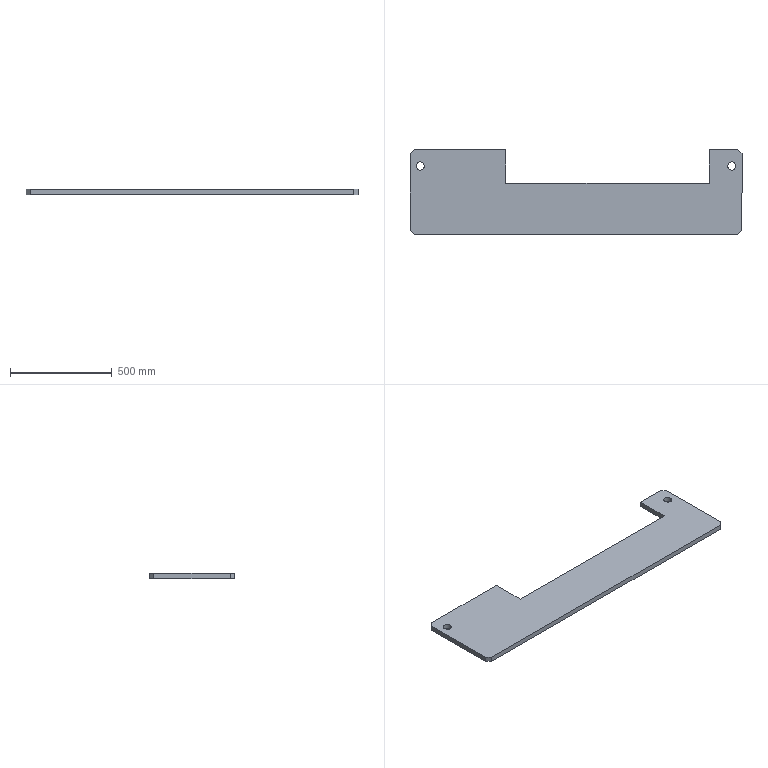Part | SolidWorks | features Chamfer 1, Extrusion 1, ICE 1 | 1 solid | 18 faces | box 1630 x 415 x 25 mm | volume 12703418 mm3 | plane 14 | cylinder 4 | commonest cylinder face diameters 40 x4
STEP:
#1=CARTESIAN_POINT('',(745.,127.5,0.));
#2=VERTEX_POINT('',#1);
#3=CARTESIAN_POINT('',(785.,127.5,0.));
#4=VERTEX_POINT('',#3);
#5=CARTESIAN_POINT('',(765.,127.5,0.));
#6=DIRECTION('',(0.,0.,1.));
#7=DIRECTION('',(1.,0.,0.));
#8=AXIS2_PLACEMENT_3D('',#5,#6,#7);
#9=CIRCLE('',#8,20.);
#10=EDGE_CURVE('',#2,#4,#9,.T.);
#11=ORIENTED_EDGE('',*,*,#10,.F.);
#12=CARTESIAN_POINT('',(745.,127.5,25.));
#13=VERTEX_POINT('',#12);
#14=CARTESIAN_POINT('',(745.,127.5,0.));
#15=DIRECTION('',(0.,0.,1.));
#16=VECTOR('',#15,1000.);
#17=LINE('',#14,#16);
#18=EDGE_CURVE('',#2,#13,#17,.T.);
#19=ORIENTED_EDGE('',*,*,#18,.T.);
#20=CARTESIAN_POINT('',(785.,127.5,25.));
#21=VERTEX_POINT('',#20);
#22=CARTESIAN_POINT('',(765.,127.5,25.));
#23=DIRECTION('',(0.,0.,-1.));
#24=DIRECTION('',(-1.,0.,0.));
#25=AXIS2_PLACEMENT_3D('',#22,#23,#24);
#26=CIRCLE('',#25,20.);
#27=EDGE_CURVE('',#21,#13,#26,.T.);
#28=ORIENTED_EDGE('',*,*,#27,.F.);
#29=CARTESIAN_POINT('',(785.,127.5,0.));
#30=DIRECTION('',(0.,0.,1.));
#31=VECTOR('',#30,1000.);
#32=LINE('',#29,#31);
#33=EDGE_CURVE('',#4,#21,#32,.T.);
#34=ORIENTED_EDGE('',*,*,#33,.F.);
#35=EDGE_LOOP('',(#11,#19,#28,#34));
#36=FACE_OUTER_BOUND('',#35,.T.);
#37=CARTESIAN_POINT('',(765.,127.5,0.));
#38=DIRECTION('',(0.,0.,1.));
#39=DIRECTION('',(1.,0.,0.));
#40=AXIS2_PLACEMENT_3D('',#37,#38,#39);
#41=CYLINDRICAL_SURFACE('',#40,20.);
#42=ADVANCED_FACE('',(#36),#41,.F.);
#43=CARTESIAN_POINT('',(-785.,127.5,0.));
#44=VERTEX_POINT('',#43);
#45=CARTESIAN_POINT('',(-745.,127.5,0.));
#46=VERTEX_POINT('',#45);
#47=CARTESIAN_POINT('',(-765.,127.5,0.));
#48=DIRECTION('',(0.,0.,1.));
#49=DIRECTION('',(1.,0.,0.));
#50=AXIS2_PLACEMENT_3D('',#47,#48,#49);
#51=CIRCLE('',#50,20.);
#52=EDGE_CURVE('',#44,#46,#51,.T.);
#53=ORIENTED_EDGE('',*,*,#52,.F.);
#54=CARTESIAN_POINT('',(-785.,127.5,25.));
#55=VERTEX_POINT('',#54);
#56=CARTESIAN_POINT('',(-785.,127.5,0.));
#57=DIRECTION('',(0.,0.,1.));
#58=VECTOR('',#57,1000.);
#59=LINE('',#56,#58);
#60=EDGE_CURVE('',#44,#55,#59,.T.);
#61=ORIENTED_EDGE('',*,*,#60,.T.);
#62=CARTESIAN_POINT('',(-745.,127.5,25.));
#63=VERTEX_POINT('',#62);
#64=CARTESIAN_POINT('',(-765.,127.5,25.));
#65=DIRECTION('',(0.,0.,-1.));
#66=DIRECTION('',(-1.,0.,0.));
#67=AXIS2_PLACEMENT_3D('',#64,#65,#66);
#68=CIRCLE('',#67,20.);
#69=EDGE_CURVE('',#63,#55,#68,.T.);
#70=ORIENTED_EDGE('',*,*,#69,.F.);
#71=CARTESIAN_POINT('',(-745.,127.5,0.));
#72=DIRECTION('',(0.,0.,1.));
#73=VECTOR('',#72,1000.);
#74=LINE('',#71,#73);
#75=EDGE_CURVE('',#46,#63,#74,.T.);
#76=ORIENTED_EDGE('',*,*,#75,.F.);
#77=EDGE_LOOP('',(#53,#61,#70,#76));
#78=FACE_OUTER_BOUND('',#77,.T.);
#79=CARTESIAN_POINT('',(-765.,127.5,0.));
#80=DIRECTION('',(0.,0.,1.));
#81=DIRECTION('',(1.,0.,0.));
#82=AXIS2_PLACEMENT_3D('',#79,#80,#81);
#83=CYLINDRICAL_SURFACE('',#82,20.);
#84=ADVANCED_FACE('',(#78),#83,.F.);
#85=CARTESIAN_POINT('',(-345.,207.5,25.));
#86=VERTEX_POINT('',#85);
#87=CARTESIAN_POINT('',(-795.,207.5,25.));
#88=VERTEX_POINT('',#87);
#89=CARTESIAN_POINT('',(815.,207.5,25.));
#90=DIRECTION('',(-1.,0.,0.));
#91=VECTOR('',#90,1000.);
#92=LINE('',#89,#91);
#93=EDGE_CURVE('',#86,#88,#92,.T.);
#94=ORIENTED_EDGE('',*,*,#93,.F.);
#95=CARTESIAN_POINT('',(-345.,207.5,0.));
#96=VERTEX_POINT('',#95);
#97=CARTESIAN_POINT('',(-345.,207.5,25.));
#98=DIRECTION('',(0.,0.,-1.));
#99=VECTOR('',#98,1000.);
#100=LINE('',#97,#99);
#101=EDGE_CURVE('',#86,#96,#100,.T.);
#102=ORIENTED_EDGE('',*,*,#101,.T.);
#103=CARTESIAN_POINT('',(-795.,207.5,0.));
#104=VERTEX_POINT('',#103);
#105=CARTESIAN_POINT('',(815.,207.5,0.));
#106=DIRECTION('',(-1.,0.,0.));
#107=VECTOR('',#106,1000.);
#108=LINE('',#105,#107);
#109=EDGE_CURVE('',#96,#104,#108,.T.);
#110=ORIENTED_EDGE('',*,*,#109,.T.);
#111=CARTESIAN_POINT('',(-795.,207.5,25.));
#112=DIRECTION('',(0.,0.,1.));
#113=VECTOR('',#112,1000.);
#114=LINE('',#111,#113);
#115=EDGE_CURVE('',#104,#88,#114,.T.);
#116=ORIENTED_EDGE('',*,*,#115,.T.);
#117=EDGE_LOOP('',(#94,#102,#110,#116));
#118=FACE_OUTER_BOUND('',#117,.T.);
#119=CARTESIAN_POINT('',(815.,207.5,25.));
#120=DIRECTION('',(0.,-1.,0.));
#121=DIRECTION('',(1.,0.,0.));
#122=AXIS2_PLACEMENT_3D('',#119,#120,#121);
#123=PLANE('',#122);
#124=ADVANCED_FACE('',(#118),#123,.F.);
#125=CARTESIAN_POINT('',(-815.,187.5,0.));
#126=VERTEX_POINT('',#125);
#127=CARTESIAN_POINT('',(-815.,-187.5,0.));
#128=VERTEX_POINT('',#127);
#129=CARTESIAN_POINT('',(-815.,207.5,0.));
#130=DIRECTION('',(0.,-1.,0.));
#131=VECTOR('',#130,1000.);
#132=LINE('',#129,#131);
#133=EDGE_CURVE('',#126,#128,#132,.T.);
#134=ORIENTED_EDGE('',*,*,#133,.T.);
#135=CARTESIAN_POINT('',(-815.,-187.5,25.));
#136=VERTEX_POINT('',#135);
#137=CARTESIAN_POINT('',(-815.,-187.5,25.));
#138=DIRECTION('',(0.,0.,1.));
#139=VECTOR('',#138,1000.);
#140=LINE('',#137,#139);
#141=EDGE_CURVE('',#128,#136,#140,.T.);
#142=ORIENTED_EDGE('',*,*,#141,.T.);
#143=CARTESIAN_POINT('',(-815.,187.5,25.));
#144=VERTEX_POINT('',#143);
#145=CARTESIAN_POINT('',(-815.,207.5,25.));
#146=DIRECTION('',(0.,-1.,0.));
#147=VECTOR('',#146,1000.);
#148=LINE('',#145,#147);
#149=EDGE_CURVE('',#144,#136,#148,.T.);
#150=ORIENTED_EDGE('',*,*,#149,.F.);
#151=CARTESIAN_POINT('',(-815.,187.5,25.));
#152=DIRECTION('',(0.,0.,-1.));
#153=VECTOR('',#152,1000.);
#154=LINE('',#151,#153);
#155=EDGE_CURVE('',#144,#126,#154,.T.);
#156=ORIENTED_EDGE('',*,*,#155,.T.);
#157=EDGE_LOOP('',(#134,#142,#150,#156));
#158=FACE_OUTER_BOUND('',#157,.T.);
#159=CARTESIAN_POINT('',(-815.,207.5,25.));
#160=DIRECTION('',(1.,0.,0.));
#161=DIRECTION('',(0.,1.,0.));
#162=AXIS2_PLACEMENT_3D('',#159,#160,#161);
#163=PLANE('',#162);
#164=ADVANCED_FACE('',(#158),#163,.F.);
#165=CARTESIAN_POINT('',(-795.,-207.5,25.));
#166=VERTEX_POINT('',#165);
#167=CARTESIAN_POINT('',(795.,-207.5,25.));
#168=VERTEX_POINT('',#167);
#169=CARTESIAN_POINT('',(815.,-207.5,25.));
#170=DIRECTION('',(1.,0.,0.));
#171=VECTOR('',#170,1000.);
#172=LINE('',#169,#171);
#173=EDGE_CURVE('',#166,#168,#172,.T.);
#174=ORIENTED_EDGE('',*,*,#173,.F.);
#175=CARTESIAN_POINT('',(-795.,-207.5,0.));
#176=VERTEX_POINT('',#175);
#177=CARTESIAN_POINT('',(-795.,-207.5,25.));
#178=DIRECTION('',(0.,0.,-1.));
#179=VECTOR('',#178,1000.);
#180=LINE('',#177,#179);
#181=EDGE_CURVE('',#166,#176,#180,.T.);
#182=ORIENTED_EDGE('',*,*,#181,.T.);
#183=CARTESIAN_POINT('',(795.,-207.5,0.));
#184=VERTEX_POINT('',#183);
#185=CARTESIAN_POINT('',(815.,-207.5,0.));
#186=DIRECTION('',(1.,0.,0.));
#187=VECTOR('',#186,1000.);
#188=LINE('',#185,#187);
#189=EDGE_CURVE('',#176,#184,#188,.T.);
#190=ORIENTED_EDGE('',*,*,#189,.T.);
#191=CARTESIAN_POINT('',(795.,-207.5,25.));
#192=DIRECTION('',(0.,0.,1.));
#193=VECTOR('',#192,1000.);
#194=LINE('',#191,#193);
#195=EDGE_CURVE('',#184,#168,#194,.T.);
#196=ORIENTED_EDGE('',*,*,#195,.T.);
#197=EDGE_LOOP('',(#174,#182,#190,#196));
#198=FACE_OUTER_BOUND('',#197,.T.);
#199=CARTESIAN_POINT('',(815.,-207.5,25.));
#200=DIRECTION('',(0.,1.,0.));
#201=DIRECTION('',(-1.,0.,0.));
#202=AXIS2_PLACEMENT_3D('',#199,#200,#201);
#203=PLANE('',#202);
#204=ADVANCED_FACE('',(#198),#203,.F.);
#205=CARTESIAN_POINT('',(815.,-187.5,25.));
#206=VERTEX_POINT('',#205);
#207=CARTESIAN_POINT('',(815.,187.5,25.));
#208=VERTEX_POINT('',#207);
#209=CARTESIAN_POINT('',(815.,207.5,25.));
#210=DIRECTION('',(0.,1.,0.));
#211=VECTOR('',#210,1000.);
#212=LINE('',#209,#211);
#213=EDGE_CURVE('',#206,#208,#212,.T.);
#214=ORIENTED_EDGE('',*,*,#213,.F.);
#215=CARTESIAN_POINT('',(815.,-187.5,0.));
#216=VERTEX_POINT('',#215);
#217=CARTESIAN_POINT('',(815.,-187.5,25.));
#218=DIRECTION('',(0.,0.,-1.));
#219=VECTOR('',#218,1000.);
#220=LINE('',#217,#219);
#221=EDGE_CURVE('',#206,#216,#220,.T.);
#222=ORIENTED_EDGE('',*,*,#221,.T.);
#223=CARTESIAN_POINT('',(815.,187.5,0.));
#224=VERTEX_POINT('',#223);
#225=CARTESIAN_POINT('',(815.,207.5,0.));
#226=DIRECTION('',(0.,1.,0.));
#227=VECTOR('',#226,1000.);
#228=LINE('',#225,#227);
#229=EDGE_CURVE('',#216,#224,#228,.T.);
#230=ORIENTED_EDGE('',*,*,#229,.T.);
#231=CARTESIAN_POINT('',(815.,187.5,25.));
#232=DIRECTION('',(0.,0.,1.));
#233=VECTOR('',#232,1000.);
#234=LINE('',#231,#233);
#235=EDGE_CURVE('',#224,#208,#234,.T.);
#236=ORIENTED_EDGE('',*,*,#235,.T.);
#237=EDGE_LOOP('',(#214,#222,#230,#236));
#238=FACE_OUTER_BOUND('',#237,.T.);
#239=CARTESIAN_POINT('',(815.,207.5,25.));
#240=DIRECTION('',(-1.,0.,0.));
#241=DIRECTION('',(0.,-1.,0.));
#242=AXIS2_PLACEMENT_3D('',#239,#240,#241);
#243=PLANE('',#242);
#244=ADVANCED_FACE('',(#238),#243,.F.);
#245=CARTESIAN_POINT('',(795.,207.5,0.));
#246=VERTEX_POINT('',#245);
#247=CARTESIAN_POINT('',(655.,207.5,0.));
#248=VERTEX_POINT('',#247);
#249=CARTESIAN_POINT('',(815.,207.5,0.));
#250=DIRECTION('',(-1.,0.,0.));
#251=VECTOR('',#250,1000.);
#252=LINE('',#249,#251);
#253=EDGE_CURVE('',#246,#248,#252,.T.);
#254=ORIENTED_EDGE('',*,*,#253,.T.);
#255=CARTESIAN_POINT('',(655.,207.5,25.));
#256=VERTEX_POINT('',#255);
#257=CARTESIAN_POINT('',(655.,207.5,25.));
#258=DIRECTION('',(0.,0.,1.));
#259=VECTOR('',#258,1000.);
#260=LINE('',#257,#259);
#261=EDGE_CURVE('',#248,#256,#260,.T.);
#262=ORIENTED_EDGE('',*,*,#261,.T.);
#263=CARTESIAN_POINT('',(795.,207.5,25.));
#264=VERTEX_POINT('',#263);
#265=CARTESIAN_POINT('',(815.,207.5,25.));
#266=DIRECTION('',(-1.,0.,0.));
#267=VECTOR('',#266,1000.);
#268=LINE('',#265,#267);
#269=EDGE_CURVE('',#264,#256,#268,.T.);
#270=ORIENTED_EDGE('',*,*,#269,.F.);
#271=CARTESIAN_POINT('',(795.,207.5,25.));
#272=DIRECTION('',(0.,0.,-1.));
#273=VECTOR('',#272,1000.);
#274=LINE('',#271,#273);
#275=EDGE_CURVE('',#264,#246,#274,.T.);
#276=ORIENTED_EDGE('',*,*,#275,.T.);
#277=EDGE_LOOP('',(#254,#262,#270,#276));
#278=FACE_OUTER_BOUND('',#277,.T.);
#279=CARTESIAN_POINT('',(815.,207.5,25.));
#280=DIRECTION('',(0.,-1.,0.));
#281=DIRECTION('',(1.,0.,0.));
#282=AXIS2_PLACEMENT_3D('',#279,#280,#281);
#283=PLANE('',#282);
#284=ADVANCED_FACE('',(#278),#283,.F.);
#285=ORIENTED_EDGE('',*,*,#27,.T.);
#286=CARTESIAN_POINT('',(765.,127.5,25.));
#287=DIRECTION('',(0.,0.,-1.));
#288=DIRECTION('',(-1.,0.,0.));
#289=AXIS2_PLACEMENT_3D('',#286,#287,#288);
#290=CIRCLE('',#289,20.);
#291=EDGE_CURVE('',#13,#21,#290,.T.);
#292=ORIENTED_EDGE('',*,*,#291,.T.);
#293=EDGE_LOOP('',(#285,#292));
#294=FACE_BOUND('',#293,.T.);
#295=ORIENTED_EDGE('',*,*,#69,.T.);
#296=CARTESIAN_POINT('',(-765.,127.5,25.));
#297=DIRECTION('',(0.,0.,-1.));
#298=DIRECTION('',(-1.,0.,0.));
#299=AXIS2_PLACEMENT_3D('',#296,#297,#298);
#300=CIRCLE('',#299,20.);
#301=EDGE_CURVE('',#55,#63,#300,.T.);
#302=ORIENTED_EDGE('',*,*,#301,.T.);
#303=EDGE_LOOP('',(#295,#302));
#304=FACE_BOUND('',#303,.T.);
#305=CARTESIAN_POINT('',(655.,42.5,25.));
#306=VERTEX_POINT('',#305);
#307=CARTESIAN_POINT('',(-345.,42.5,25.));
#308=VERTEX_POINT('',#307);
#309=CARTESIAN_POINT('',(0.,42.5,25.));
#310=DIRECTION('',(-1.,0.,0.));
#311=VECTOR('',#310,1000.);
#312=LINE('',#309,#311);
#313=EDGE_CURVE('',#306,#308,#312,.T.);
#314=ORIENTED_EDGE('',*,*,#313,.T.);
#315=CARTESIAN_POINT('',(-345.,0.,25.));
#316=DIRECTION('',(0.,1.,0.));
#317=VECTOR('',#316,1000.);
#318=LINE('',#315,#317);
#319=EDGE_CURVE('',#308,#86,#318,.T.);
#320=ORIENTED_EDGE('',*,*,#319,.T.);
#321=ORIENTED_EDGE('',*,*,#93,.T.);
#322=CARTESIAN_POINT('',(-815.,187.5,25.));
#323=DIRECTION('',(-0.7071,-0.7071,0.));
#324=VECTOR('',#323,1000.);
#325=LINE('',#322,#324);
#326=EDGE_CURVE('',#88,#144,#325,.T.);
#327=ORIENTED_EDGE('',*,*,#326,.T.);
#328=ORIENTED_EDGE('',*,*,#149,.T.);
#329=CARTESIAN_POINT('',(-795.,-207.5,25.));
#330=DIRECTION('',(0.7071,-0.7071,0.));
#331=VECTOR('',#330,1000.);
#332=LINE('',#329,#331);
#333=EDGE_CURVE('',#136,#166,#332,.T.);
#334=ORIENTED_EDGE('',*,*,#333,.T.);
#335=ORIENTED_EDGE('',*,*,#173,.T.);
#336=CARTESIAN_POINT('',(815.,-187.5,25.));
#337=DIRECTION('',(0.7071,0.7071,0.));
#338=VECTOR('',#337,1000.);
#339=LINE('',#336,#338);
#340=EDGE_CURVE('',#168,#206,#339,.T.);
#341=ORIENTED_EDGE('',*,*,#340,.T.);
#342=ORIENTED_EDGE('',*,*,#213,.T.);
#343=CARTESIAN_POINT('',(795.,207.5,25.));
#344=DIRECTION('',(-0.7071,0.7071,0.));
#345=VECTOR('',#344,1000.);
#346=LINE('',#343,#345);
#347=EDGE_CURVE('',#208,#264,#346,.T.);
#348=ORIENTED_EDGE('',*,*,#347,.T.);
#349=ORIENTED_EDGE('',*,*,#269,.T.);
#350=CARTESIAN_POINT('',(655.,0.,25.));
#351=DIRECTION('',(0.,-1.,0.));
#352=VECTOR('',#351,1000.);
#353=LINE('',#350,#352);
#354=EDGE_CURVE('',#256,#306,#353,.T.);
#355=ORIENTED_EDGE('',*,*,#354,.T.);
#356=EDGE_LOOP('',(#314,#320,#321,#327,#328,#334,#335,#341,#342,#348,#349,#355));
#357=FACE_OUTER_BOUND('',#356,.T.);
#358=CARTESIAN_POINT('',(0.,0.,25.));
#359=DIRECTION('',(0.,0.,-1.));
#360=DIRECTION('',(-1.,0.,0.));
#361=AXIS2_PLACEMENT_3D('',#358,#359,#360);
#362=PLANE('',#361);
#363=ADVANCED_FACE('',(#294,#304,#357),#362,.F.);
#364=CARTESIAN_POINT('',(765.,127.5,0.));
#365=DIRECTION('',(0.,0.,1.));
#366=DIRECTION('',(1.,0.,0.));
#367=AXIS2_PLACEMENT_3D('',#364,#365,#366);
#368=CIRCLE('',#367,20.);
#369=EDGE_CURVE('',#4,#2,#368,.T.);
#370=ORIENTED_EDGE('',*,*,#369,.T.);
#371=ORIENTED_EDGE('',*,*,#10,.T.);
#372=EDGE_LOOP('',(#370,#371));
#373=FACE_BOUND('',#372,.T.);
#374=CARTESIAN_POINT('',(-765.,127.5,0.));
#375=DIRECTION('',(0.,0.,1.));
#376=DIRECTION('',(1.,0.,0.));
#377=AXIS2_PLACEMENT_3D('',#374,#375,#376);
#378=CIRCLE('',#377,20.);
#379=EDGE_CURVE('',#46,#44,#378,.T.);
#380=ORIENTED_EDGE('',*,*,#379,.T.);
#381=ORIENTED_EDGE('',*,*,#52,.T.);
#382=EDGE_LOOP('',(#380,#381));
#383=FACE_BOUND('',#382,.T.);
#384=CARTESIAN_POINT('',(-345.,42.5,0.));
#385=VERTEX_POINT('',#384);
#386=CARTESIAN_POINT('',(-345.,0.,0.));
#387=DIRECTION('',(0.,1.,0.));
#388=VECTOR('',#387,1000.);
#389=LINE('',#386,#388);
#390=EDGE_CURVE('',#385,#96,#389,.T.);
#391=ORIENTED_EDGE('',*,*,#390,.F.);
#392=CARTESIAN_POINT('',(655.,42.5,0.));
#393=VERTEX_POINT('',#392);
#394=CARTESIAN_POINT('',(-345.,42.5,0.));
#395=DIRECTION('',(1.,0.,0.));
#396=VECTOR('',#395,1000.);
#397=LINE('',#394,#396);
#398=EDGE_CURVE('',#385,#393,#397,.T.);
#399=ORIENTED_EDGE('',*,*,#398,.T.);
#400=CARTESIAN_POINT('',(655.,42.5,0.));
#401=DIRECTION('',(0.,1.,0.));
#402=VECTOR('',#401,1000.);
#403=LINE('',#400,#402);
#404=EDGE_CURVE('',#393,#248,#403,.T.);
#405=ORIENTED_EDGE('',*,*,#404,.T.);
#406=ORIENTED_EDGE('',*,*,#253,.F.);
#407=CARTESIAN_POINT('',(501.25,501.25,0.));
#408=DIRECTION('',(0.7071,-0.7071,0.));
#409=VECTOR('',#408,1000.);
#410=LINE('',#407,#409);
#411=EDGE_CURVE('',#246,#224,#410,.T.);
#412=ORIENTED_EDGE('',*,*,#411,.T.);
#413=ORIENTED_EDGE('',*,*,#229,.F.);
#414=CARTESIAN_POINT('',(501.25,-501.25,0.));
#415=DIRECTION('',(-0.7071,-0.7071,0.));
#416=VECTOR('',#415,1000.);
#417=LINE('',#414,#416);
#418=EDGE_CURVE('',#216,#184,#417,.T.);
#419=ORIENTED_EDGE('',*,*,#418,.T.);
#420=ORIENTED_EDGE('',*,*,#189,.F.);
#421=CARTESIAN_POINT('',(-501.25,-501.25,0.));
#422=DIRECTION('',(-0.7071,0.7071,0.));
#423=VECTOR('',#422,1000.);
#424=LINE('',#421,#423);
#425=EDGE_CURVE('',#176,#128,#424,.T.);
#426=ORIENTED_EDGE('',*,*,#425,.T.);
#427=ORIENTED_EDGE('',*,*,#133,.F.);
#428=CARTESIAN_POINT('',(-501.25,501.25,0.));
#429=DIRECTION('',(0.7071,0.7071,0.));
#430=VECTOR('',#429,1000.);
#431=LINE('',#428,#430);
#432=EDGE_CURVE('',#126,#104,#431,.T.);
#433=ORIENTED_EDGE('',*,*,#432,.T.);
#434=ORIENTED_EDGE('',*,*,#109,.F.);
#435=EDGE_LOOP('',(#391,#399,#405,#406,#412,#413,#419,#420,#426,#427,#433,#434));
#436=FACE_OUTER_BOUND('',#435,.T.);
#437=CARTESIAN_POINT('',(0.,0.,0.));
#438=DIRECTION('',(0.,0.,-1.));
#439=DIRECTION('',(-1.,0.,0.));
#440=AXIS2_PLACEMENT_3D('',#437,#438,#439);
#441=PLANE('',#440);
#442=ADVANCED_FACE('',(#373,#383,#436),#441,.T.);
#443=ORIENTED_EDGE('',*,*,#333,.F.);
#444=ORIENTED_EDGE('',*,*,#141,.F.);
#445=ORIENTED_EDGE('',*,*,#425,.F.);
#446=ORIENTED_EDGE('',*,*,#181,.F.);
#447=EDGE_LOOP('',(#443,#444,#445,#446));
#448=FACE_OUTER_BOUND('',#447,.T.);
#449=CARTESIAN_POINT('',(-795.,-207.5,25.));
#450=DIRECTION('',(0.7071,0.7071,0.));
#451=DIRECTION('',(0.,0.,-1.));
#452=AXIS2_PLACEMENT_3D('',#449,#450,#451);
#453=PLANE('',#452);
#454=ADVANCED_FACE('',(#448),#453,.F.);
#455=ORIENTED_EDGE('',*,*,#340,.F.);
#456=ORIENTED_EDGE('',*,*,#195,.F.);
#457=ORIENTED_EDGE('',*,*,#418,.F.);
#458=ORIENTED_EDGE('',*,*,#221,.F.);
#459=EDGE_LOOP('',(#455,#456,#457,#458));
#460=FACE_OUTER_BOUND('',#459,.T.);
#461=CARTESIAN_POINT('',(815.,-187.5,25.));
#462=DIRECTION('',(-0.7071,0.7071,0.));
#463=DIRECTION('',(0.,0.,-1.));
#464=AXIS2_PLACEMENT_3D('',#461,#462,#463);
#465=PLANE('',#464);
#466=ADVANCED_FACE('',(#460),#465,.F.);
#467=ORIENTED_EDGE('',*,*,#347,.F.);
#468=ORIENTED_EDGE('',*,*,#235,.F.);
#469=ORIENTED_EDGE('',*,*,#411,.F.);
#470=ORIENTED_EDGE('',*,*,#275,.F.);
#471=EDGE_LOOP('',(#467,#468,#469,#470));
#472=FACE_OUTER_BOUND('',#471,.T.);
#473=CARTESIAN_POINT('',(795.,207.5,25.));
#474=DIRECTION('',(-0.7071,-0.7071,0.));
#475=DIRECTION('',(0.,0.,-1.));
#476=AXIS2_PLACEMENT_3D('',#473,#474,#475);
#477=PLANE('',#476);
#478=ADVANCED_FACE('',(#472),#477,.F.);
#479=ORIENTED_EDGE('',*,*,#326,.F.);
#480=ORIENTED_EDGE('',*,*,#115,.F.);
#481=ORIENTED_EDGE('',*,*,#432,.F.);
#482=ORIENTED_EDGE('',*,*,#155,.F.);
#483=EDGE_LOOP('',(#479,#480,#481,#482));
#484=FACE_OUTER_BOUND('',#483,.T.);
#485=CARTESIAN_POINT('',(-815.,187.5,25.));
#486=DIRECTION('',(0.7071,-0.7071,0.));
#487=DIRECTION('',(0.,0.,-1.));
#488=AXIS2_PLACEMENT_3D('',#485,#486,#487);
#489=PLANE('',#488);
#490=ADVANCED_FACE('',(#484),#489,.F.);
#491=ORIENTED_EDGE('',*,*,#319,.F.);
#492=CARTESIAN_POINT('',(-345.,42.5,0.));
#493=DIRECTION('',(0.,0.,1.));
#494=VECTOR('',#493,1000.);
#495=LINE('',#492,#494);
#496=EDGE_CURVE('',#385,#308,#495,.T.);
#497=ORIENTED_EDGE('',*,*,#496,.F.);
#498=ORIENTED_EDGE('',*,*,#390,.T.);
#499=ORIENTED_EDGE('',*,*,#101,.F.);
#500=EDGE_LOOP('',(#491,#497,#498,#499));
#501=FACE_OUTER_BOUND('',#500,.T.);
#502=CARTESIAN_POINT('',(-345.,42.5,0.));
#503=DIRECTION('',(-1.,0.,0.));
#504=DIRECTION('',(0.,0.,1.));
#505=AXIS2_PLACEMENT_3D('',#502,#503,#504);
#506=PLANE('',#505);
#507=ADVANCED_FACE('',(#501),#506,.F.);
#508=ORIENTED_EDGE('',*,*,#404,.F.);
#509=CARTESIAN_POINT('',(655.,42.5,0.));
#510=DIRECTION('',(0.,0.,1.));
#511=VECTOR('',#510,1000.);
#512=LINE('',#509,#511);
#513=EDGE_CURVE('',#393,#306,#512,.T.);
#514=ORIENTED_EDGE('',*,*,#513,.T.);
#515=ORIENTED_EDGE('',*,*,#354,.F.);
#516=ORIENTED_EDGE('',*,*,#261,.F.);
#517=EDGE_LOOP('',(#508,#514,#515,#516));
#518=FACE_OUTER_BOUND('',#517,.T.);
#519=CARTESIAN_POINT('',(655.,42.5,0.));
#520=DIRECTION('',(1.,0.,0.));
#521=DIRECTION('',(0.,0.,-1.));
#522=AXIS2_PLACEMENT_3D('',#519,#520,#521);
#523=PLANE('',#522);
#524=ADVANCED_FACE('',(#518),#523,.F.);
#525=ORIENTED_EDGE('',*,*,#513,.F.);
#526=ORIENTED_EDGE('',*,*,#398,.F.);
#527=ORIENTED_EDGE('',*,*,#496,.T.);
#528=ORIENTED_EDGE('',*,*,#313,.F.);
#529=EDGE_LOOP('',(#525,#526,#527,#528));
#530=FACE_OUTER_BOUND('',#529,.T.);
#531=CARTESIAN_POINT('',(-345.,42.5,0.));
#532=DIRECTION('',(0.,-1.,0.));
#533=DIRECTION('',(0.,0.,-1.));
#534=AXIS2_PLACEMENT_3D('',#531,#532,#533);
#535=PLANE('',#534);
#536=ADVANCED_FACE('',(#530),#535,.F.);
#537=ORIENTED_EDGE('',*,*,#60,.F.);
#538=ORIENTED_EDGE('',*,*,#379,.F.);
#539=ORIENTED_EDGE('',*,*,#75,.T.);
#540=ORIENTED_EDGE('',*,*,#301,.F.);
#541=EDGE_LOOP('',(#537,#538,#539,#540));
#542=FACE_OUTER_BOUND('',#541,.T.);
#543=CARTESIAN_POINT('',(-765.,127.5,0.));
#544=DIRECTION('',(0.,0.,1.));
#545=DIRECTION('',(1.,0.,0.));
#546=AXIS2_PLACEMENT_3D('',#543,#544,#545);
#547=CYLINDRICAL_SURFACE('',#546,20.);
#548=ADVANCED_FACE('',(#542),#547,.F.);
#549=ORIENTED_EDGE('',*,*,#18,.F.);
#550=ORIENTED_EDGE('',*,*,#369,.F.);
#551=ORIENTED_EDGE('',*,*,#33,.T.);
#552=ORIENTED_EDGE('',*,*,#291,.F.);
#553=EDGE_LOOP('',(#549,#550,#551,#552));
#554=FACE_OUTER_BOUND('',#553,.T.);
#555=CARTESIAN_POINT('',(765.,127.5,0.));
#556=DIRECTION('',(0.,0.,1.));
#557=DIRECTION('',(1.,0.,0.));
#558=AXIS2_PLACEMENT_3D('',#555,#556,#557);
#559=CYLINDRICAL_SURFACE('',#558,20.);
#560=ADVANCED_FACE('',(#554),#559,.F.);
#561=CLOSED_SHELL('',(#42,#84,#124,#164,#204,#244,#284,#363,#442,#454,#466,#478,#490,#507,#524,#536,#548,#560));
#562=MANIFOLD_SOLID_BREP('',#561);
#563=CARTESIAN_POINT('',(0.,0.,0.));
#564=DIRECTION('',(0.,0.,1.));
#565=DIRECTION('',(1.,0.,0.));
#566=AXIS2_PLACEMENT_3D('',#563,#564,#565);
#567=(LENGTH_UNIT()NAMED_UNIT(*)SI_UNIT(.MILLI.,.METRE.));
#568=UNCERTAINTY_MEASURE_WITH_UNIT(LENGTH_MEASURE(0.00001),#567,'','');
#569=(NAMED_UNIT(*)PLANE_ANGLE_UNIT()SI_UNIT($,.RADIAN.));
#570=(NAMED_UNIT(*)SI_UNIT($,.STERADIAN.)SOLID_ANGLE_UNIT());
#571=(GEOMETRIC_REPRESENTATION_CONTEXT(3)GLOBAL_UNCERTAINTY_ASSIGNED_CONTEXT((#568))GLOBAL_UNIT_ASSIGNED_CONTEXT((#567,#569,#570))REPRESENTATION_CONTEXT('',''));
#572=ADVANCED_BREP_SHAPE_REPRESENTATION('',(#562,#566),#571);